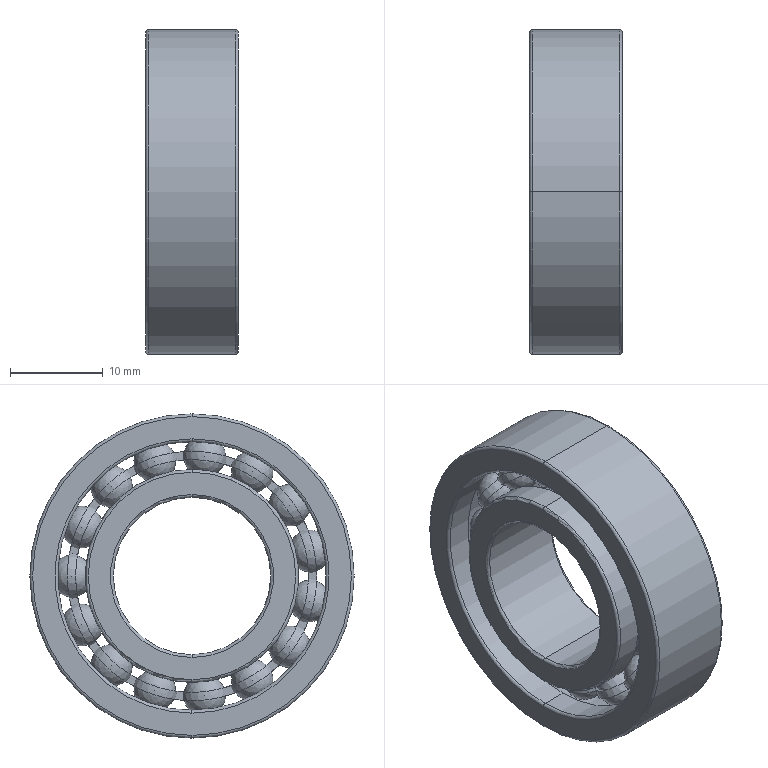Part | SolidWorks | 17 solids | 188 faces | box 10 x 35 x 35 mm | volume 5427 mm3 | cylinder 70 | sphere 62 | plane 34 | torus 22 | commonest cylinder face diameters 25.1 x29 26.9 x29 23 x4 29 x4 17 x2 35 x2